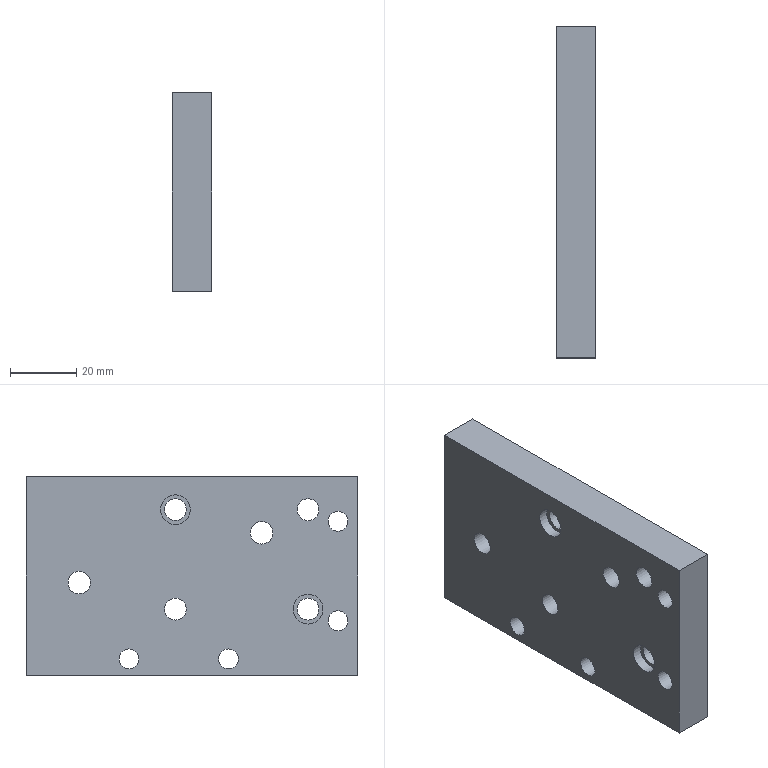Part | NX | features BREP 1 | 1 solid | 30 faces | box 12 x 100 x 60 mm | volume 66744 mm3 | cylinder 17 | plane 12 | cone 1 | commonest cylinder face diameters 6 x4 6.6 x4 11 x4 6.8 x2 9 x2 3.3 x1
STEP:
#1=CARTESIAN_POINT('',(1.4,-35.,-13.3));
#2=VERTEX_POINT('',#1);
#3=CARTESIAN_POINT('',(1.4,-35.,-10.));
#4=DIRECTION('',(1.,0.,0.));
#5=DIRECTION('',(0.,0.,-1.));
#6=AXIS2_PLACEMENT_3D('',#3,#4,#5);
#7=CIRCLE('',#6,3.3);
#8=EDGE_CURVE('',#2,#2,#7,.T.);
#9=ORIENTED_EDGE('',*,*,#8,.T.);
#10=EDGE_LOOP('',(#9));
#11=FACE_BOUND('',#10,.T.);
#12=CARTESIAN_POINT('',(-3.,-35.,-6.7));
#13=VERTEX_POINT('',#12);
#14=CARTESIAN_POINT('',(-3.,-35.,-10.));
#15=DIRECTION('',(1.,0.,0.));
#16=DIRECTION('',(0.,0.,1.));
#17=AXIS2_PLACEMENT_3D('',#14,#15,#16);
#18=CIRCLE('',#17,3.3);
#19=EDGE_CURVE('',#13,#13,#18,.T.);
#20=ORIENTED_EDGE('',*,*,#19,.F.);
#21=EDGE_LOOP('',(#20));
#22=FACE_BOUND('',#21,.T.);
#23=CARTESIAN_POINT('',(6.,-35.,-10.));
#24=DIRECTION('',(1.,0.,0.));
#25=DIRECTION('',(0.,0.,1.));
#26=AXIS2_PLACEMENT_3D('',#23,#24,#25);
#27=CYLINDRICAL_SURFACE('',#26,3.3);
#28=ADVANCED_FACE('',(#11,#22),#27,.F.);
#29=CARTESIAN_POINT('',(1.4,5.,16.7));
#30=VERTEX_POINT('',#29);
#31=CARTESIAN_POINT('',(1.4,5.,20.));
#32=DIRECTION('',(1.,0.,0.));
#33=DIRECTION('',(0.,0.,-1.));
#34=AXIS2_PLACEMENT_3D('',#31,#32,#33);
#35=CIRCLE('',#34,3.3);
#36=EDGE_CURVE('',#30,#30,#35,.T.);
#37=ORIENTED_EDGE('',*,*,#36,.T.);
#38=EDGE_LOOP('',(#37));
#39=FACE_BOUND('',#38,.T.);
#40=CARTESIAN_POINT('',(-3.,5.,23.3));
#41=VERTEX_POINT('',#40);
#42=CARTESIAN_POINT('',(-3.,5.,20.));
#43=DIRECTION('',(1.,0.,0.));
#44=DIRECTION('',(0.,0.,1.));
#45=AXIS2_PLACEMENT_3D('',#42,#43,#44);
#46=CIRCLE('',#45,3.3);
#47=EDGE_CURVE('',#41,#41,#46,.T.);
#48=ORIENTED_EDGE('',*,*,#47,.F.);
#49=EDGE_LOOP('',(#48));
#50=FACE_BOUND('',#49,.T.);
#51=CARTESIAN_POINT('',(6.,5.,20.));
#52=DIRECTION('',(1.,0.,0.));
#53=DIRECTION('',(0.,0.,1.));
#54=AXIS2_PLACEMENT_3D('',#51,#52,#53);
#55=CYLINDRICAL_SURFACE('',#54,3.3);
#56=ADVANCED_FACE('',(#39,#50),#55,.F.);
#57=CARTESIAN_POINT('',(-6.,-50.,-30.));
#58=VERTEX_POINT('',#57);
#59=CARTESIAN_POINT('',(-6.,50.,-30.));
#60=VERTEX_POINT('',#59);
#61=CARTESIAN_POINT('',(-6.,-50.,-30.));
#62=DIRECTION('',(0.,1.,0.));
#63=VECTOR('',#62,1000.);
#64=LINE('',#61,#63);
#65=EDGE_CURVE('',#58,#60,#64,.T.);
#66=ORIENTED_EDGE('',*,*,#65,.T.);
#67=CARTESIAN_POINT('',(6.,50.,-30.));
#68=VERTEX_POINT('',#67);
#69=CARTESIAN_POINT('',(6.,50.,-30.));
#70=DIRECTION('',(-1.,0.,0.));
#71=VECTOR('',#70,1000.);
#72=LINE('',#69,#71);
#73=EDGE_CURVE('',#68,#60,#72,.T.);
#74=ORIENTED_EDGE('',*,*,#73,.F.);
#75=CARTESIAN_POINT('',(6.,-50.,-30.));
#76=VERTEX_POINT('',#75);
#77=CARTESIAN_POINT('',(6.,-50.,-30.));
#78=DIRECTION('',(0.,1.,0.));
#79=VECTOR('',#78,1000.);
#80=LINE('',#77,#79);
#81=EDGE_CURVE('',#76,#68,#80,.T.);
#82=ORIENTED_EDGE('',*,*,#81,.F.);
#83=CARTESIAN_POINT('',(6.,-50.,-30.));
#84=DIRECTION('',(-1.,0.,0.));
#85=VECTOR('',#84,1000.);
#86=LINE('',#83,#85);
#87=EDGE_CURVE('',#76,#58,#86,.T.);
#88=ORIENTED_EDGE('',*,*,#87,.T.);
#89=EDGE_LOOP('',(#66,#74,#82,#88));
#90=FACE_BOUND('',#89,.T.);
#91=CARTESIAN_POINT('',(6.,-50.,-30.));
#92=DIRECTION('',(0.,0.,1.));
#93=DIRECTION('',(-1.,0.,0.));
#94=AXIS2_PLACEMENT_3D('',#91,#92,#93);
#95=PLANE('',#94);
#96=ADVANCED_FACE('',(#90),#95,.F.);
#97=CARTESIAN_POINT('',(0.,50.,11.65));
#98=VERTEX_POINT('',#97);
#99=CARTESIAN_POINT('',(0.,50.,10.));
#100=DIRECTION('',(0.,1.,0.));
#101=DIRECTION('',(0.,0.,1.));
#102=AXIS2_PLACEMENT_3D('',#99,#100,#101);
#103=CIRCLE('',#102,1.65);
#104=EDGE_CURVE('',#98,#98,#103,.T.);
#105=ORIENTED_EDGE('',*,*,#104,.F.);
#106=EDGE_LOOP('',(#105));
#107=FACE_BOUND('',#106,.T.);
#108=CARTESIAN_POINT('',(-6.,50.,30.));
#109=VERTEX_POINT('',#108);
#110=CARTESIAN_POINT('',(-6.,50.,30.));
#111=DIRECTION('',(0.,0.,1.));
#112=VECTOR('',#111,1000.);
#113=LINE('',#110,#112);
#114=EDGE_CURVE('',#60,#109,#113,.T.);
#115=ORIENTED_EDGE('',*,*,#114,.T.);
#116=CARTESIAN_POINT('',(6.,50.,30.));
#117=VERTEX_POINT('',#116);
#118=CARTESIAN_POINT('',(6.,50.,30.));
#119=DIRECTION('',(-1.,0.,0.));
#120=VECTOR('',#119,1000.);
#121=LINE('',#118,#120);
#122=EDGE_CURVE('',#117,#109,#121,.T.);
#123=ORIENTED_EDGE('',*,*,#122,.F.);
#124=CARTESIAN_POINT('',(6.,50.,30.));
#125=DIRECTION('',(0.,0.,1.));
#126=VECTOR('',#125,1000.);
#127=LINE('',#124,#126);
#128=EDGE_CURVE('',#68,#117,#127,.T.);
#129=ORIENTED_EDGE('',*,*,#128,.F.);
#130=ORIENTED_EDGE('',*,*,#73,.T.);
#131=EDGE_LOOP('',(#115,#123,#129,#130));
#132=FACE_BOUND('',#131,.T.);
#133=CARTESIAN_POINT('',(6.,50.,30.));
#134=DIRECTION('',(0.,-1.,0.));
#135=DIRECTION('',(0.,0.,1.));
#136=AXIS2_PLACEMENT_3D('',#133,#134,#135);
#137=PLANE('',#136);
#138=ADVANCED_FACE('',(#107,#132),#137,.F.);
#139=CARTESIAN_POINT('',(-6.,-50.,30.));
#140=VERTEX_POINT('',#139);
#141=CARTESIAN_POINT('',(-6.,-50.,30.));
#142=DIRECTION('',(0.,-1.,0.));
#143=VECTOR('',#142,1000.);
#144=LINE('',#141,#143);
#145=EDGE_CURVE('',#109,#140,#144,.T.);
#146=ORIENTED_EDGE('',*,*,#145,.T.);
#147=CARTESIAN_POINT('',(6.,-50.,30.));
#148=VERTEX_POINT('',#147);
#149=CARTESIAN_POINT('',(6.,-50.,30.));
#150=DIRECTION('',(-1.,0.,0.));
#151=VECTOR('',#150,1000.);
#152=LINE('',#149,#151);
#153=EDGE_CURVE('',#148,#140,#152,.T.);
#154=ORIENTED_EDGE('',*,*,#153,.F.);
#155=CARTESIAN_POINT('',(6.,-50.,30.));
#156=DIRECTION('',(0.,-1.,0.));
#157=VECTOR('',#156,1000.);
#158=LINE('',#155,#157);
#159=EDGE_CURVE('',#117,#148,#158,.T.);
#160=ORIENTED_EDGE('',*,*,#159,.F.);
#161=ORIENTED_EDGE('',*,*,#122,.T.);
#162=EDGE_LOOP('',(#146,#154,#160,#161));
#163=FACE_BOUND('',#162,.T.);
#164=CARTESIAN_POINT('',(6.,-50.,30.));
#165=DIRECTION('',(0.,0.,-1.));
#166=DIRECTION('',(1.,0.,0.));
#167=AXIS2_PLACEMENT_3D('',#164,#165,#166);
#168=PLANE('',#167);
#169=ADVANCED_FACE('',(#163),#168,.F.);
#170=CARTESIAN_POINT('',(-6.,-50.,30.));
#171=DIRECTION('',(0.,0.,-1.));
#172=VECTOR('',#171,1000.);
#173=LINE('',#170,#172);
#174=EDGE_CURVE('',#140,#58,#173,.T.);
#175=ORIENTED_EDGE('',*,*,#174,.T.);
#176=ORIENTED_EDGE('',*,*,#87,.F.);
#177=CARTESIAN_POINT('',(6.,-50.,30.));
#178=DIRECTION('',(0.,0.,-1.));
#179=VECTOR('',#178,1000.);
#180=LINE('',#177,#179);
#181=EDGE_CURVE('',#148,#76,#180,.T.);
#182=ORIENTED_EDGE('',*,*,#181,.F.);
#183=ORIENTED_EDGE('',*,*,#153,.T.);
#184=EDGE_LOOP('',(#175,#176,#182,#183));
#185=FACE_BOUND('',#184,.T.);
#186=CARTESIAN_POINT('',(6.,-50.,30.));
#187=DIRECTION('',(0.,1.,0.));
#188=DIRECTION('',(0.,0.,-1.));
#189=AXIS2_PLACEMENT_3D('',#186,#187,#188);
#190=PLANE('',#189);
#191=ADVANCED_FACE('',(#185),#190,.F.);
#192=CARTESIAN_POINT('',(6.,19.,-28.));
#193=VERTEX_POINT('',#192);
#194=CARTESIAN_POINT('',(6.,19.,-25.));
#195=DIRECTION('',(1.,0.,0.));
#196=DIRECTION('',(0.,0.,-1.));
#197=AXIS2_PLACEMENT_3D('',#194,#195,#196);
#198=CIRCLE('',#197,3.);
#199=EDGE_CURVE('',#193,#193,#198,.T.);
#200=ORIENTED_EDGE('',*,*,#199,.F.);
#201=EDGE_LOOP('',(#200));
#202=FACE_BOUND('',#201,.T.);
#203=CARTESIAN_POINT('',(6.,-11.,-28.));
#204=VERTEX_POINT('',#203);
#205=CARTESIAN_POINT('',(6.,-11.,-25.));
#206=DIRECTION('',(1.,0.,0.));
#207=DIRECTION('',(0.,0.,-1.));
#208=AXIS2_PLACEMENT_3D('',#205,#206,#207);
#209=CIRCLE('',#208,3.);
#210=EDGE_CURVE('',#204,#204,#209,.T.);
#211=ORIENTED_EDGE('',*,*,#210,.F.);
#212=EDGE_LOOP('',(#211));
#213=FACE_BOUND('',#212,.T.);
#214=CARTESIAN_POINT('',(6.,-44.,-16.5));
#215=VERTEX_POINT('',#214);
#216=CARTESIAN_POINT('',(6.,-44.,-13.5));
#217=DIRECTION('',(1.,0.,0.));
#218=DIRECTION('',(0.,0.,-1.));
#219=AXIS2_PLACEMENT_3D('',#216,#217,#218);
#220=CIRCLE('',#219,3.);
#221=EDGE_CURVE('',#215,#215,#220,.T.);
#222=ORIENTED_EDGE('',*,*,#221,.F.);
#223=EDGE_LOOP('',(#222));
#224=FACE_BOUND('',#223,.T.);
#225=CARTESIAN_POINT('',(6.,-44.,13.5));
#226=VERTEX_POINT('',#225);
#227=CARTESIAN_POINT('',(6.,-44.,16.5));
#228=DIRECTION('',(1.,0.,0.));
#229=DIRECTION('',(0.,0.,-1.));
#230=AXIS2_PLACEMENT_3D('',#227,#228,#229);
#231=CIRCLE('',#230,3.);
#232=EDGE_CURVE('',#226,#226,#231,.T.);
#233=ORIENTED_EDGE('',*,*,#232,.F.);
#234=EDGE_LOOP('',(#233));
#235=FACE_BOUND('',#234,.T.);
#236=CARTESIAN_POINT('',(6.,34.,-5.4));
#237=VERTEX_POINT('',#236);
#238=CARTESIAN_POINT('',(6.,34.,-2.));
#239=DIRECTION('',(1.,0.,0.));
#240=DIRECTION('',(0.,0.,-1.));
#241=AXIS2_PLACEMENT_3D('',#238,#239,#240);
#242=CIRCLE('',#241,3.4);
#243=EDGE_CURVE('',#237,#237,#242,.T.);
#244=ORIENTED_EDGE('',*,*,#243,.F.);
#245=EDGE_LOOP('',(#244));
#246=FACE_BOUND('',#245,.T.);
#247=CARTESIAN_POINT('',(6.,-21.,9.6));
#248=VERTEX_POINT('',#247);
#249=CARTESIAN_POINT('',(6.,-21.,13.));
#250=DIRECTION('',(1.,0.,0.));
#251=DIRECTION('',(0.,0.,-1.));
#252=AXIS2_PLACEMENT_3D('',#249,#250,#251);
#253=CIRCLE('',#252,3.4);
#254=EDGE_CURVE('',#248,#248,#253,.T.);
#255=ORIENTED_EDGE('',*,*,#254,.F.);
#256=EDGE_LOOP('',(#255));
#257=FACE_BOUND('',#256,.T.);
#258=CARTESIAN_POINT('',(6.,5.,14.5));
#259=VERTEX_POINT('',#258);
#260=CARTESIAN_POINT('',(6.,5.,20.));
#261=DIRECTION('',(1.,0.,0.));
#262=DIRECTION('',(0.,0.,-1.));
#263=AXIS2_PLACEMENT_3D('',#260,#261,#262);
#264=CIRCLE('',#263,5.5);
#265=EDGE_CURVE('',#259,#259,#264,.T.);
#266=ORIENTED_EDGE('',*,*,#265,.F.);
#267=EDGE_LOOP('',(#266));
#268=FACE_BOUND('',#267,.T.);
#269=CARTESIAN_POINT('',(6.,-35.,-15.5));
#270=VERTEX_POINT('',#269);
#271=CARTESIAN_POINT('',(6.,-35.,-10.));
#272=DIRECTION('',(1.,0.,0.));
#273=DIRECTION('',(0.,0.,-1.));
#274=AXIS2_PLACEMENT_3D('',#271,#272,#273);
#275=CIRCLE('',#274,5.5);
#276=EDGE_CURVE('',#270,#270,#275,.T.);
#277=ORIENTED_EDGE('',*,*,#276,.F.);
#278=EDGE_LOOP('',(#277));
#279=FACE_BOUND('',#278,.T.);
#280=CARTESIAN_POINT('',(6.,-35.,14.5));
#281=VERTEX_POINT('',#280);
#282=CARTESIAN_POINT('',(6.,-35.,20.));
#283=DIRECTION('',(1.,0.,0.));
#284=DIRECTION('',(0.,0.,-1.));
#285=AXIS2_PLACEMENT_3D('',#282,#283,#284);
#286=CIRCLE('',#285,5.5);
#287=EDGE_CURVE('',#281,#281,#286,.T.);
#288=ORIENTED_EDGE('',*,*,#287,.F.);
#289=EDGE_LOOP('',(#288));
#290=FACE_BOUND('',#289,.T.);
#291=CARTESIAN_POINT('',(6.,5.,-15.5));
#292=VERTEX_POINT('',#291);
#293=CARTESIAN_POINT('',(6.,5.,-10.));
#294=DIRECTION('',(1.,0.,0.));
#295=DIRECTION('',(0.,0.,-1.));
#296=AXIS2_PLACEMENT_3D('',#293,#294,#295);
#297=CIRCLE('',#296,5.5);
#298=EDGE_CURVE('',#292,#292,#297,.T.);
#299=ORIENTED_EDGE('',*,*,#298,.F.);
#300=EDGE_LOOP('',(#299));
#301=FACE_BOUND('',#300,.T.);
#302=ORIENTED_EDGE('',*,*,#81,.T.);
#303=ORIENTED_EDGE('',*,*,#128,.T.);
#304=ORIENTED_EDGE('',*,*,#159,.T.);
#305=ORIENTED_EDGE('',*,*,#181,.T.);
#306=EDGE_LOOP('',(#302,#303,#304,#305));
#307=FACE_BOUND('',#306,.T.);
#308=CARTESIAN_POINT('',(6.,0.,0.));
#309=DIRECTION('',(-1.,0.,0.));
#310=DIRECTION('',(0.,0.,-1.));
#311=AXIS2_PLACEMENT_3D('',#308,#309,#310);
#312=PLANE('',#311);
#313=ADVANCED_FACE('',(#202,#213,#224,#235,#246,#257,#268,#279,#290,#301,#307),#312,.F.);
#314=CARTESIAN_POINT('',(-6.,19.,-28.));
#315=VERTEX_POINT('',#314);
#316=CARTESIAN_POINT('',(-6.,19.,-25.));
#317=DIRECTION('',(1.,0.,0.));
#318=DIRECTION('',(0.,0.,-1.));
#319=AXIS2_PLACEMENT_3D('',#316,#317,#318);
#320=CIRCLE('',#319,3.);
#321=EDGE_CURVE('',#315,#315,#320,.T.);
#322=ORIENTED_EDGE('',*,*,#321,.T.);
#323=EDGE_LOOP('',(#322));
#324=FACE_BOUND('',#323,.T.);
#325=CARTESIAN_POINT('',(-6.,-11.,-28.));
#326=VERTEX_POINT('',#325);
#327=CARTESIAN_POINT('',(-6.,-11.,-25.));
#328=DIRECTION('',(1.,0.,0.));
#329=DIRECTION('',(0.,0.,-1.));
#330=AXIS2_PLACEMENT_3D('',#327,#328,#329);
#331=CIRCLE('',#330,3.);
#332=EDGE_CURVE('',#326,#326,#331,.T.);
#333=ORIENTED_EDGE('',*,*,#332,.T.);
#334=EDGE_LOOP('',(#333));
#335=FACE_BOUND('',#334,.T.);
#336=CARTESIAN_POINT('',(-6.,-44.,-16.5));
#337=VERTEX_POINT('',#336);
#338=CARTESIAN_POINT('',(-6.,-44.,-13.5));
#339=DIRECTION('',(1.,0.,0.));
#340=DIRECTION('',(0.,0.,-1.));
#341=AXIS2_PLACEMENT_3D('',#338,#339,#340);
#342=CIRCLE('',#341,3.);
#343=EDGE_CURVE('',#337,#337,#342,.T.);
#344=ORIENTED_EDGE('',*,*,#343,.T.);
#345=EDGE_LOOP('',(#344));
#346=FACE_BOUND('',#345,.T.);
#347=CARTESIAN_POINT('',(-6.,-44.,13.5));
#348=VERTEX_POINT('',#347);
#349=CARTESIAN_POINT('',(-6.,-44.,16.5));
#350=DIRECTION('',(1.,0.,0.));
#351=DIRECTION('',(0.,0.,-1.));
#352=AXIS2_PLACEMENT_3D('',#349,#350,#351);
#353=CIRCLE('',#352,3.);
#354=EDGE_CURVE('',#348,#348,#353,.T.);
#355=ORIENTED_EDGE('',*,*,#354,.T.);
#356=EDGE_LOOP('',(#355));
#357=FACE_BOUND('',#356,.T.);
#358=CARTESIAN_POINT('',(-6.,34.,-5.4));
#359=VERTEX_POINT('',#358);
#360=CARTESIAN_POINT('',(-6.,34.,-2.));
#361=DIRECTION('',(1.,0.,0.));
#362=DIRECTION('',(0.,0.,-1.));
#363=AXIS2_PLACEMENT_3D('',#360,#361,#362);
#364=CIRCLE('',#363,3.4);
#365=EDGE_CURVE('',#359,#359,#364,.T.);
#366=ORIENTED_EDGE('',*,*,#365,.T.);
#367=EDGE_LOOP('',(#366));
#368=FACE_BOUND('',#367,.T.);
#369=CARTESIAN_POINT('',(-6.,-21.,9.6));
#370=VERTEX_POINT('',#369);
#371=CARTESIAN_POINT('',(-6.,-21.,13.));
#372=DIRECTION('',(1.,0.,0.));
#373=DIRECTION('',(0.,0.,-1.));
#374=AXIS2_PLACEMENT_3D('',#371,#372,#373);
#375=CIRCLE('',#374,3.4);
#376=EDGE_CURVE('',#370,#370,#375,.T.);
#377=ORIENTED_EDGE('',*,*,#376,.T.);
#378=EDGE_LOOP('',(#377));
#379=FACE_BOUND('',#378,.T.);
#380=CARTESIAN_POINT('',(-6.,5.,24.5));
#381=VERTEX_POINT('',#380);
#382=CARTESIAN_POINT('',(-6.,5.,20.));
#383=DIRECTION('',(-1.,0.,0.));
#384=DIRECTION('',(0.,0.,1.));
#385=AXIS2_PLACEMENT_3D('',#382,#383,#384);
#386=CIRCLE('',#385,4.5);
#387=EDGE_CURVE('',#381,#381,#386,.T.);
#388=ORIENTED_EDGE('',*,*,#387,.F.);
#389=EDGE_LOOP('',(#388));
#390=FACE_BOUND('',#389,.T.);
#391=CARTESIAN_POINT('',(-6.,-35.,-5.5));
#392=VERTEX_POINT('',#391);
#393=CARTESIAN_POINT('',(-6.,-35.,-10.));
#394=DIRECTION('',(-1.,0.,0.));
#395=DIRECTION('',(0.,0.,1.));
#396=AXIS2_PLACEMENT_3D('',#393,#394,#395);
#397=CIRCLE('',#396,4.5);
#398=EDGE_CURVE('',#392,#392,#397,.T.);
#399=ORIENTED_EDGE('',*,*,#398,.F.);
#400=EDGE_LOOP('',(#399));
#401=FACE_BOUND('',#400,.T.);
#402=CARTESIAN_POINT('',(-6.,-35.,16.7));
#403=VERTEX_POINT('',#402);
#404=CARTESIAN_POINT('',(-6.,-35.,20.));
#405=DIRECTION('',(1.,0.,0.));
#406=DIRECTION('',(0.,0.,-1.));
#407=AXIS2_PLACEMENT_3D('',#404,#405,#406);
#408=CIRCLE('',#407,3.3);
#409=EDGE_CURVE('',#403,#403,#408,.T.);
#410=ORIENTED_EDGE('',*,*,#409,.T.);
#411=EDGE_LOOP('',(#410));
#412=FACE_BOUND('',#411,.T.);
#413=CARTESIAN_POINT('',(-6.,5.,-13.3));
#414=VERTEX_POINT('',#413);
#415=CARTESIAN_POINT('',(-6.,5.,-10.));
#416=DIRECTION('',(1.,0.,0.));
#417=DIRECTION('',(0.,0.,-1.));
#418=AXIS2_PLACEMENT_3D('',#415,#416,#417);
#419=CIRCLE('',#418,3.3);
#420=EDGE_CURVE('',#414,#414,#419,.T.);
#421=ORIENTED_EDGE('',*,*,#420,.T.);
#422=EDGE_LOOP('',(#421));
#423=FACE_BOUND('',#422,.T.);
#424=ORIENTED_EDGE('',*,*,#65,.F.);
#425=ORIENTED_EDGE('',*,*,#174,.F.);
#426=ORIENTED_EDGE('',*,*,#145,.F.);
#427=ORIENTED_EDGE('',*,*,#114,.F.);
#428=EDGE_LOOP('',(#424,#425,#426,#427));
#429=FACE_BOUND('',#428,.T.);
#430=CARTESIAN_POINT('',(-6.,0.,0.));
#431=DIRECTION('',(-1.,0.,0.));
#432=DIRECTION('',(0.,0.,-1.));
#433=AXIS2_PLACEMENT_3D('',#430,#431,#432);
#434=PLANE('',#433);
#435=ADVANCED_FACE('',(#324,#335,#346,#357,#368,#379,#390,#401,#412,#423,#429),#434,.T.);
#436=ORIENTED_EDGE('',*,*,#420,.F.);
#437=EDGE_LOOP('',(#436));
#438=FACE_BOUND('',#437,.T.);
#439=CARTESIAN_POINT('',(1.4,5.,-13.3));
#440=VERTEX_POINT('',#439);
#441=CARTESIAN_POINT('',(1.4,5.,-10.));
#442=DIRECTION('',(1.,0.,0.));
#443=DIRECTION('',(0.,0.,-1.));
#444=AXIS2_PLACEMENT_3D('',#441,#442,#443);
#445=CIRCLE('',#444,3.3);
#446=EDGE_CURVE('',#440,#440,#445,.T.);
#447=ORIENTED_EDGE('',*,*,#446,.T.);
#448=EDGE_LOOP('',(#447));
#449=FACE_BOUND('',#448,.T.);
#450=CARTESIAN_POINT('',(6.,5.,-10.));
#451=DIRECTION('',(1.,0.,0.));
#452=DIRECTION('',(0.,0.,1.));
#453=AXIS2_PLACEMENT_3D('',#450,#451,#452);
#454=CYLINDRICAL_SURFACE('',#453,3.3);
#455=ADVANCED_FACE('',(#438,#449),#454,.F.);
#456=ORIENTED_EDGE('',*,*,#446,.F.);
#457=EDGE_LOOP('',(#456));
#458=FACE_BOUND('',#457,.T.);
#459=CARTESIAN_POINT('',(1.4,5.,-15.5));
#460=VERTEX_POINT('',#459);
#461=CARTESIAN_POINT('',(1.4,5.,-10.));
#462=DIRECTION('',(1.,0.,0.));
#463=DIRECTION('',(0.,0.,-1.));
#464=AXIS2_PLACEMENT_3D('',#461,#462,#463);
#465=CIRCLE('',#464,5.5);
#466=EDGE_CURVE('',#460,#460,#465,.T.);
#467=ORIENTED_EDGE('',*,*,#466,.T.);
#468=EDGE_LOOP('',(#467));
#469=FACE_BOUND('',#468,.T.);
#470=CARTESIAN_POINT('',(1.4,8.3,-10.));
#471=DIRECTION('',(-1.,0.,0.));
#472=DIRECTION('',(0.,0.,-1.));
#473=AXIS2_PLACEMENT_3D('',#470,#471,#472);
#474=PLANE('',#473);
#475=ADVANCED_FACE('',(#458,#469),#474,.F.);
#476=ORIENTED_EDGE('',*,*,#466,.F.);
#477=EDGE_LOOP('',(#476));
#478=FACE_BOUND('',#477,.T.);
#479=ORIENTED_EDGE('',*,*,#298,.T.);
#480=EDGE_LOOP('',(#479));
#481=FACE_BOUND('',#480,.T.);
#482=CARTESIAN_POINT('',(6.,5.,-10.));
#483=DIRECTION('',(1.,0.,0.));
#484=DIRECTION('',(0.,0.,1.));
#485=AXIS2_PLACEMENT_3D('',#482,#483,#484);
#486=CYLINDRICAL_SURFACE('',#485,5.5);
#487=ADVANCED_FACE('',(#478,#481),#486,.F.);
#488=ORIENTED_EDGE('',*,*,#409,.F.);
#489=EDGE_LOOP('',(#488));
#490=FACE_BOUND('',#489,.T.);
#491=CARTESIAN_POINT('',(1.4,-35.,16.7));
#492=VERTEX_POINT('',#491);
#493=CARTESIAN_POINT('',(1.4,-35.,20.));
#494=DIRECTION('',(1.,0.,0.));
#495=DIRECTION('',(0.,0.,-1.));
#496=AXIS2_PLACEMENT_3D('',#493,#494,#495);
#497=CIRCLE('',#496,3.3);
#498=EDGE_CURVE('',#492,#492,#497,.T.);
#499=ORIENTED_EDGE('',*,*,#498,.T.);
#500=EDGE_LOOP('',(#499));
#501=FACE_BOUND('',#500,.T.);
#502=CARTESIAN_POINT('',(6.,-35.,20.));
#503=DIRECTION('',(1.,0.,0.));
#504=DIRECTION('',(0.,0.,1.));
#505=AXIS2_PLACEMENT_3D('',#502,#503,#504);
#506=CYLINDRICAL_SURFACE('',#505,3.3);
#507=ADVANCED_FACE('',(#490,#501),#506,.F.);
#508=ORIENTED_EDGE('',*,*,#498,.F.);
#509=EDGE_LOOP('',(#508));
#510=FACE_BOUND('',#509,.T.);
#511=CARTESIAN_POINT('',(1.4,-35.,14.5));
#512=VERTEX_POINT('',#511);
#513=CARTESIAN_POINT('',(1.4,-35.,20.));
#514=DIRECTION('',(1.,0.,0.));
#515=DIRECTION('',(0.,0.,-1.));
#516=AXIS2_PLACEMENT_3D('',#513,#514,#515);
#517=CIRCLE('',#516,5.5);
#518=EDGE_CURVE('',#512,#512,#517,.T.);
#519=ORIENTED_EDGE('',*,*,#518,.T.);
#520=EDGE_LOOP('',(#519));
#521=FACE_BOUND('',#520,.T.);
#522=CARTESIAN_POINT('',(1.4,-31.7,20.));
#523=DIRECTION('',(-1.,0.,0.));
#524=DIRECTION('',(0.,0.,-1.));
#525=AXIS2_PLACEMENT_3D('',#522,#523,#524);
#526=PLANE('',#525);
#527=ADVANCED_FACE('',(#510,#521),#526,.F.);
#528=ORIENTED_EDGE('',*,*,#518,.F.);
#529=EDGE_LOOP('',(#528));
#530=FACE_BOUND('',#529,.T.);
#531=ORIENTED_EDGE('',*,*,#287,.T.);
#532=EDGE_LOOP('',(#531));
#533=FACE_BOUND('',#532,.T.);
#534=CARTESIAN_POINT('',(6.,-35.,20.));
#535=DIRECTION('',(1.,0.,0.));
#536=DIRECTION('',(0.,0.,1.));
#537=AXIS2_PLACEMENT_3D('',#534,#535,#536);
#538=CYLINDRICAL_SURFACE('',#537,5.5);
#539=ADVANCED_FACE('',(#530,#533),#538,.F.);
#540=ORIENTED_EDGE('',*,*,#8,.F.);
#541=EDGE_LOOP('',(#540));
#542=FACE_BOUND('',#541,.T.);
#543=CARTESIAN_POINT('',(1.4,-35.,-15.5));
#544=VERTEX_POINT('',#543);
#545=CARTESIAN_POINT('',(1.4,-35.,-10.));
#546=DIRECTION('',(1.,0.,0.));
#547=DIRECTION('',(0.,0.,-1.));
#548=AXIS2_PLACEMENT_3D('',#545,#546,#547);
#549=CIRCLE('',#548,5.5);
#550=EDGE_CURVE('',#544,#544,#549,.T.);
#551=ORIENTED_EDGE('',*,*,#550,.T.);
#552=EDGE_LOOP('',(#551));
#553=FACE_BOUND('',#552,.T.);
#554=CARTESIAN_POINT('',(1.4,-31.7,-10.));
#555=DIRECTION('',(-1.,0.,0.));
#556=DIRECTION('',(0.,0.,-1.));
#557=AXIS2_PLACEMENT_3D('',#554,#555,#556);
#558=PLANE('',#557);
#559=ADVANCED_FACE('',(#542,#553),#558,.F.);
#560=ORIENTED_EDGE('',*,*,#550,.F.);
#561=EDGE_LOOP('',(#560));
#562=FACE_BOUND('',#561,.T.);
#563=ORIENTED_EDGE('',*,*,#276,.T.);
#564=EDGE_LOOP('',(#563));
#565=FACE_BOUND('',#564,.T.);
#566=CARTESIAN_POINT('',(6.,-35.,-10.));
#567=DIRECTION('',(1.,0.,0.));
#568=DIRECTION('',(0.,0.,1.));
#569=AXIS2_PLACEMENT_3D('',#566,#567,#568);
#570=CYLINDRICAL_SURFACE('',#569,5.5);
#571=ADVANCED_FACE('',(#562,#565),#570,.F.);
#572=ORIENTED_EDGE('',*,*,#36,.F.);
#573=EDGE_LOOP('',(#572));
#574=FACE_BOUND('',#573,.T.);
#575=CARTESIAN_POINT('',(1.4,5.,14.5));
#576=VERTEX_POINT('',#575);
#577=CARTESIAN_POINT('',(1.4,5.,20.));
#578=DIRECTION('',(1.,0.,0.));
#579=DIRECTION('',(0.,0.,-1.));
#580=AXIS2_PLACEMENT_3D('',#577,#578,#579);
#581=CIRCLE('',#580,5.5);
#582=EDGE_CURVE('',#576,#576,#581,.T.);
#583=ORIENTED_EDGE('',*,*,#582,.T.);
#584=EDGE_LOOP('',(#583));
#585=FACE_BOUND('',#584,.T.);
#586=CARTESIAN_POINT('',(1.4,8.3,20.));
#587=DIRECTION('',(-1.,0.,0.));
#588=DIRECTION('',(0.,0.,-1.));
#589=AXIS2_PLACEMENT_3D('',#586,#587,#588);
#590=PLANE('',#589);
#591=ADVANCED_FACE('',(#574,#585),#590,.F.);
#592=ORIENTED_EDGE('',*,*,#582,.F.);
#593=EDGE_LOOP('',(#592));
#594=FACE_BOUND('',#593,.T.);
#595=ORIENTED_EDGE('',*,*,#265,.T.);
#596=EDGE_LOOP('',(#595));
#597=FACE_BOUND('',#596,.T.);
#598=CARTESIAN_POINT('',(6.,5.,20.));
#599=DIRECTION('',(1.,0.,0.));
#600=DIRECTION('',(0.,0.,1.));
#601=AXIS2_PLACEMENT_3D('',#598,#599,#600);
#602=CYLINDRICAL_SURFACE('',#601,5.5);
#603=ADVANCED_FACE('',(#594,#597),#602,.F.);
#604=CARTESIAN_POINT('',(-3.,5.,24.5));
#605=VERTEX_POINT('',#604);
#606=CARTESIAN_POINT('',(-3.,5.,20.));
#607=DIRECTION('',(-1.,0.,0.));
#608=DIRECTION('',(0.,0.,1.));
#609=AXIS2_PLACEMENT_3D('',#606,#607,#608);
#610=CIRCLE('',#609,4.5);
#611=EDGE_CURVE('',#605,#605,#610,.T.);
#612=ORIENTED_EDGE('',*,*,#611,.T.);
#613=EDGE_LOOP('',(#612));
#614=FACE_BOUND('',#613,.T.);
#615=ORIENTED_EDGE('',*,*,#47,.T.);
#616=EDGE_LOOP('',(#615));
#617=FACE_BOUND('',#616,.T.);
#618=CARTESIAN_POINT('',(-3.,5.,20.));
#619=DIRECTION('',(-1.,0.,0.));
#620=DIRECTION('',(0.,0.,-1.));
#621=AXIS2_PLACEMENT_3D('',#618,#619,#620);
#622=PLANE('',#621);
#623=ADVANCED_FACE('',(#614,#617),#622,.T.);
#624=ORIENTED_EDGE('',*,*,#611,.F.);
#625=EDGE_LOOP('',(#624));
#626=FACE_BOUND('',#625,.T.);
#627=ORIENTED_EDGE('',*,*,#387,.T.);
#628=EDGE_LOOP('',(#627));
#629=FACE_BOUND('',#628,.T.);
#630=CARTESIAN_POINT('',(-3.,5.,20.));
#631=DIRECTION('',(-1.,0.,0.));
#632=DIRECTION('',(0.,0.,-1.));
#633=AXIS2_PLACEMENT_3D('',#630,#631,#632);
#634=CYLINDRICAL_SURFACE('',#633,4.5);
#635=ADVANCED_FACE('',(#626,#629),#634,.F.);
#636=CARTESIAN_POINT('',(-3.,-35.,-5.5));
#637=VERTEX_POINT('',#636);
#638=CARTESIAN_POINT('',(-3.,-35.,-10.));
#639=DIRECTION('',(-1.,0.,0.));
#640=DIRECTION('',(0.,0.,1.));
#641=AXIS2_PLACEMENT_3D('',#638,#639,#640);
#642=CIRCLE('',#641,4.5);
#643=EDGE_CURVE('',#637,#637,#642,.T.);
#644=ORIENTED_EDGE('',*,*,#643,.T.);
#645=EDGE_LOOP('',(#644));
#646=FACE_BOUND('',#645,.T.);
#647=ORIENTED_EDGE('',*,*,#19,.T.);
#648=EDGE_LOOP('',(#647));
#649=FACE_BOUND('',#648,.T.);
#650=CARTESIAN_POINT('',(-3.,-35.,-10.));
#651=DIRECTION('',(-1.,0.,0.));
#652=DIRECTION('',(0.,0.,-1.));
#653=AXIS2_PLACEMENT_3D('',#650,#651,#652);
#654=PLANE('',#653);
#655=ADVANCED_FACE('',(#646,#649),#654,.T.);
#656=ORIENTED_EDGE('',*,*,#643,.F.);
#657=EDGE_LOOP('',(#656));
#658=FACE_BOUND('',#657,.T.);
#659=ORIENTED_EDGE('',*,*,#398,.T.);
#660=EDGE_LOOP('',(#659));
#661=FACE_BOUND('',#660,.T.);
#662=CARTESIAN_POINT('',(-3.,-35.,-10.));
#663=DIRECTION('',(-1.,0.,0.));
#664=DIRECTION('',(0.,0.,-1.));
#665=AXIS2_PLACEMENT_3D('',#662,#663,#664);
#666=CYLINDRICAL_SURFACE('',#665,4.5);
#667=ADVANCED_FACE('',(#658,#661),#666,.F.);
#668=ORIENTED_EDGE('',*,*,#376,.F.);
#669=EDGE_LOOP('',(#668));
#670=FACE_BOUND('',#669,.T.);
#671=ORIENTED_EDGE('',*,*,#254,.T.);
#672=EDGE_LOOP('',(#671));
#673=FACE_BOUND('',#672,.T.);
#674=CARTESIAN_POINT('',(6.,-21.,13.));
#675=DIRECTION('',(1.,0.,0.));
#676=DIRECTION('',(0.,0.,1.));
#677=AXIS2_PLACEMENT_3D('',#674,#675,#676);
#678=CYLINDRICAL_SURFACE('',#677,3.4);
#679=ADVANCED_FACE('',(#670,#673),#678,.F.);
#680=ORIENTED_EDGE('',*,*,#365,.F.);
#681=EDGE_LOOP('',(#680));
#682=FACE_BOUND('',#681,.T.);
#683=ORIENTED_EDGE('',*,*,#243,.T.);
#684=EDGE_LOOP('',(#683));
#685=FACE_BOUND('',#684,.T.);
#686=CARTESIAN_POINT('',(6.,34.,-2.));
#687=DIRECTION('',(1.,0.,0.));
#688=DIRECTION('',(0.,0.,1.));
#689=AXIS2_PLACEMENT_3D('',#686,#687,#688);
#690=CYLINDRICAL_SURFACE('',#689,3.4);
#691=ADVANCED_FACE('',(#682,#685),#690,.F.);
#692=ORIENTED_EDGE('',*,*,#354,.F.);
#693=EDGE_LOOP('',(#692));
#694=FACE_BOUND('',#693,.T.);
#695=ORIENTED_EDGE('',*,*,#232,.T.);
#696=EDGE_LOOP('',(#695));
#697=FACE_BOUND('',#696,.T.);
#698=CARTESIAN_POINT('',(6.,-44.,16.5));
#699=DIRECTION('',(1.,0.,0.));
#700=DIRECTION('',(0.,0.,1.));
#701=AXIS2_PLACEMENT_3D('',#698,#699,#700);
#702=CYLINDRICAL_SURFACE('',#701,3.);
#703=ADVANCED_FACE('',(#694,#697),#702,.F.);
#704=ORIENTED_EDGE('',*,*,#343,.F.);
#705=EDGE_LOOP('',(#704));
#706=FACE_BOUND('',#705,.T.);
#707=ORIENTED_EDGE('',*,*,#221,.T.);
#708=EDGE_LOOP('',(#707));
#709=FACE_BOUND('',#708,.T.);
#710=CARTESIAN_POINT('',(6.,-44.,-13.5));
#711=DIRECTION('',(1.,0.,0.));
#712=DIRECTION('',(0.,0.,1.));
#713=AXIS2_PLACEMENT_3D('',#710,#711,#712);
#714=CYLINDRICAL_SURFACE('',#713,3.);
#715=ADVANCED_FACE('',(#706,#709),#714,.F.);
#716=ORIENTED_EDGE('',*,*,#332,.F.);
#717=EDGE_LOOP('',(#716));
#718=FACE_BOUND('',#717,.T.);
#719=ORIENTED_EDGE('',*,*,#210,.T.);
#720=EDGE_LOOP('',(#719));
#721=FACE_BOUND('',#720,.T.);
#722=CARTESIAN_POINT('',(6.,-11.,-25.));
#723=DIRECTION('',(1.,0.,0.));
#724=DIRECTION('',(0.,0.,1.));
#725=AXIS2_PLACEMENT_3D('',#722,#723,#724);
#726=CYLINDRICAL_SURFACE('',#725,3.);
#727=ADVANCED_FACE('',(#718,#721),#726,.F.);
#728=ORIENTED_EDGE('',*,*,#321,.F.);
#729=EDGE_LOOP('',(#728));
#730=FACE_BOUND('',#729,.T.);
#731=ORIENTED_EDGE('',*,*,#199,.T.);
#732=EDGE_LOOP('',(#731));
#733=FACE_BOUND('',#732,.T.);
#734=CARTESIAN_POINT('',(6.,19.,-25.));
#735=DIRECTION('',(1.,0.,0.));
#736=DIRECTION('',(0.,0.,1.));
#737=AXIS2_PLACEMENT_3D('',#734,#735,#736);
#738=CYLINDRICAL_SURFACE('',#737,3.);
#739=ADVANCED_FACE('',(#730,#733),#738,.F.);
#740=CARTESIAN_POINT('',(0.,38.909,10.));
#741=VERTEX_POINT('',#740);
#742=VERTEX_LOOP('',#741);
#743=FACE_BOUND('',#742,.T.);
#744=CARTESIAN_POINT('',(0.,39.9,11.65));
#745=VERTEX_POINT('',#744);
#746=CARTESIAN_POINT('',(0.,39.9,10.));
#747=DIRECTION('',(0.,1.,0.));
#748=DIRECTION('',(0.,0.,1.));
#749=AXIS2_PLACEMENT_3D('',#746,#747,#748);
#750=CIRCLE('',#749,1.65);
#751=EDGE_CURVE('',#745,#745,#750,.T.);
#752=ORIENTED_EDGE('',*,*,#751,.T.);
#753=EDGE_LOOP('',(#752));
#754=FACE_BOUND('',#753,.T.);
#755=CARTESIAN_POINT('',(0.,39.9,10.));
#756=DIRECTION('',(0.,1.,0.));
#757=DIRECTION('',(0.,0.,-1.));
#758=AXIS2_PLACEMENT_3D('',#755,#756,#757);
#759=CONICAL_SURFACE('',#758,1.65,1.03);
#760=ADVANCED_FACE('',(#743,#754),#759,.F.);
#761=ORIENTED_EDGE('',*,*,#751,.F.);
#762=EDGE_LOOP('',(#761));
#763=FACE_BOUND('',#762,.T.);
#764=ORIENTED_EDGE('',*,*,#104,.T.);
#765=EDGE_LOOP('',(#764));
#766=FACE_BOUND('',#765,.T.);
#767=CARTESIAN_POINT('',(0.,50.,10.));
#768=DIRECTION('',(0.,1.,0.));
#769=DIRECTION('',(0.,0.,-1.));
#770=AXIS2_PLACEMENT_3D('',#767,#768,#769);
#771=CYLINDRICAL_SURFACE('',#770,1.65);
#772=ADVANCED_FACE('',(#763,#766),#771,.F.);
#773=CLOSED_SHELL('',(#28,#56,#96,#138,#169,#191,#313,#435,#455,#475,#487,#507,#527,#539,#559,#571,#591,#603,#623,#635,#655,#667,#679,#691,#703,#715,#727,#739,#760,#772));
#774=MANIFOLD_SOLID_BREP('',#773);
#775=(LENGTH_UNIT()NAMED_UNIT(*)SI_UNIT(.MILLI.,.METRE.));
#776=UNCERTAINTY_MEASURE_WITH_UNIT(LENGTH_MEASURE(0.00001),#775,'','');
#777=(NAMED_UNIT(*)PLANE_ANGLE_UNIT()SI_UNIT($,.RADIAN.));
#778=(NAMED_UNIT(*)SI_UNIT($,.STERADIAN.)SOLID_ANGLE_UNIT());
#779=(GEOMETRIC_REPRESENTATION_CONTEXT(3)GLOBAL_UNCERTAINTY_ASSIGNED_CONTEXT((#776))GLOBAL_UNIT_ASSIGNED_CONTEXT((#775,#777,#778))REPRESENTATION_CONTEXT('',''));
#780=ADVANCED_BREP_SHAPE_REPRESENTATION('',(#774),#779);